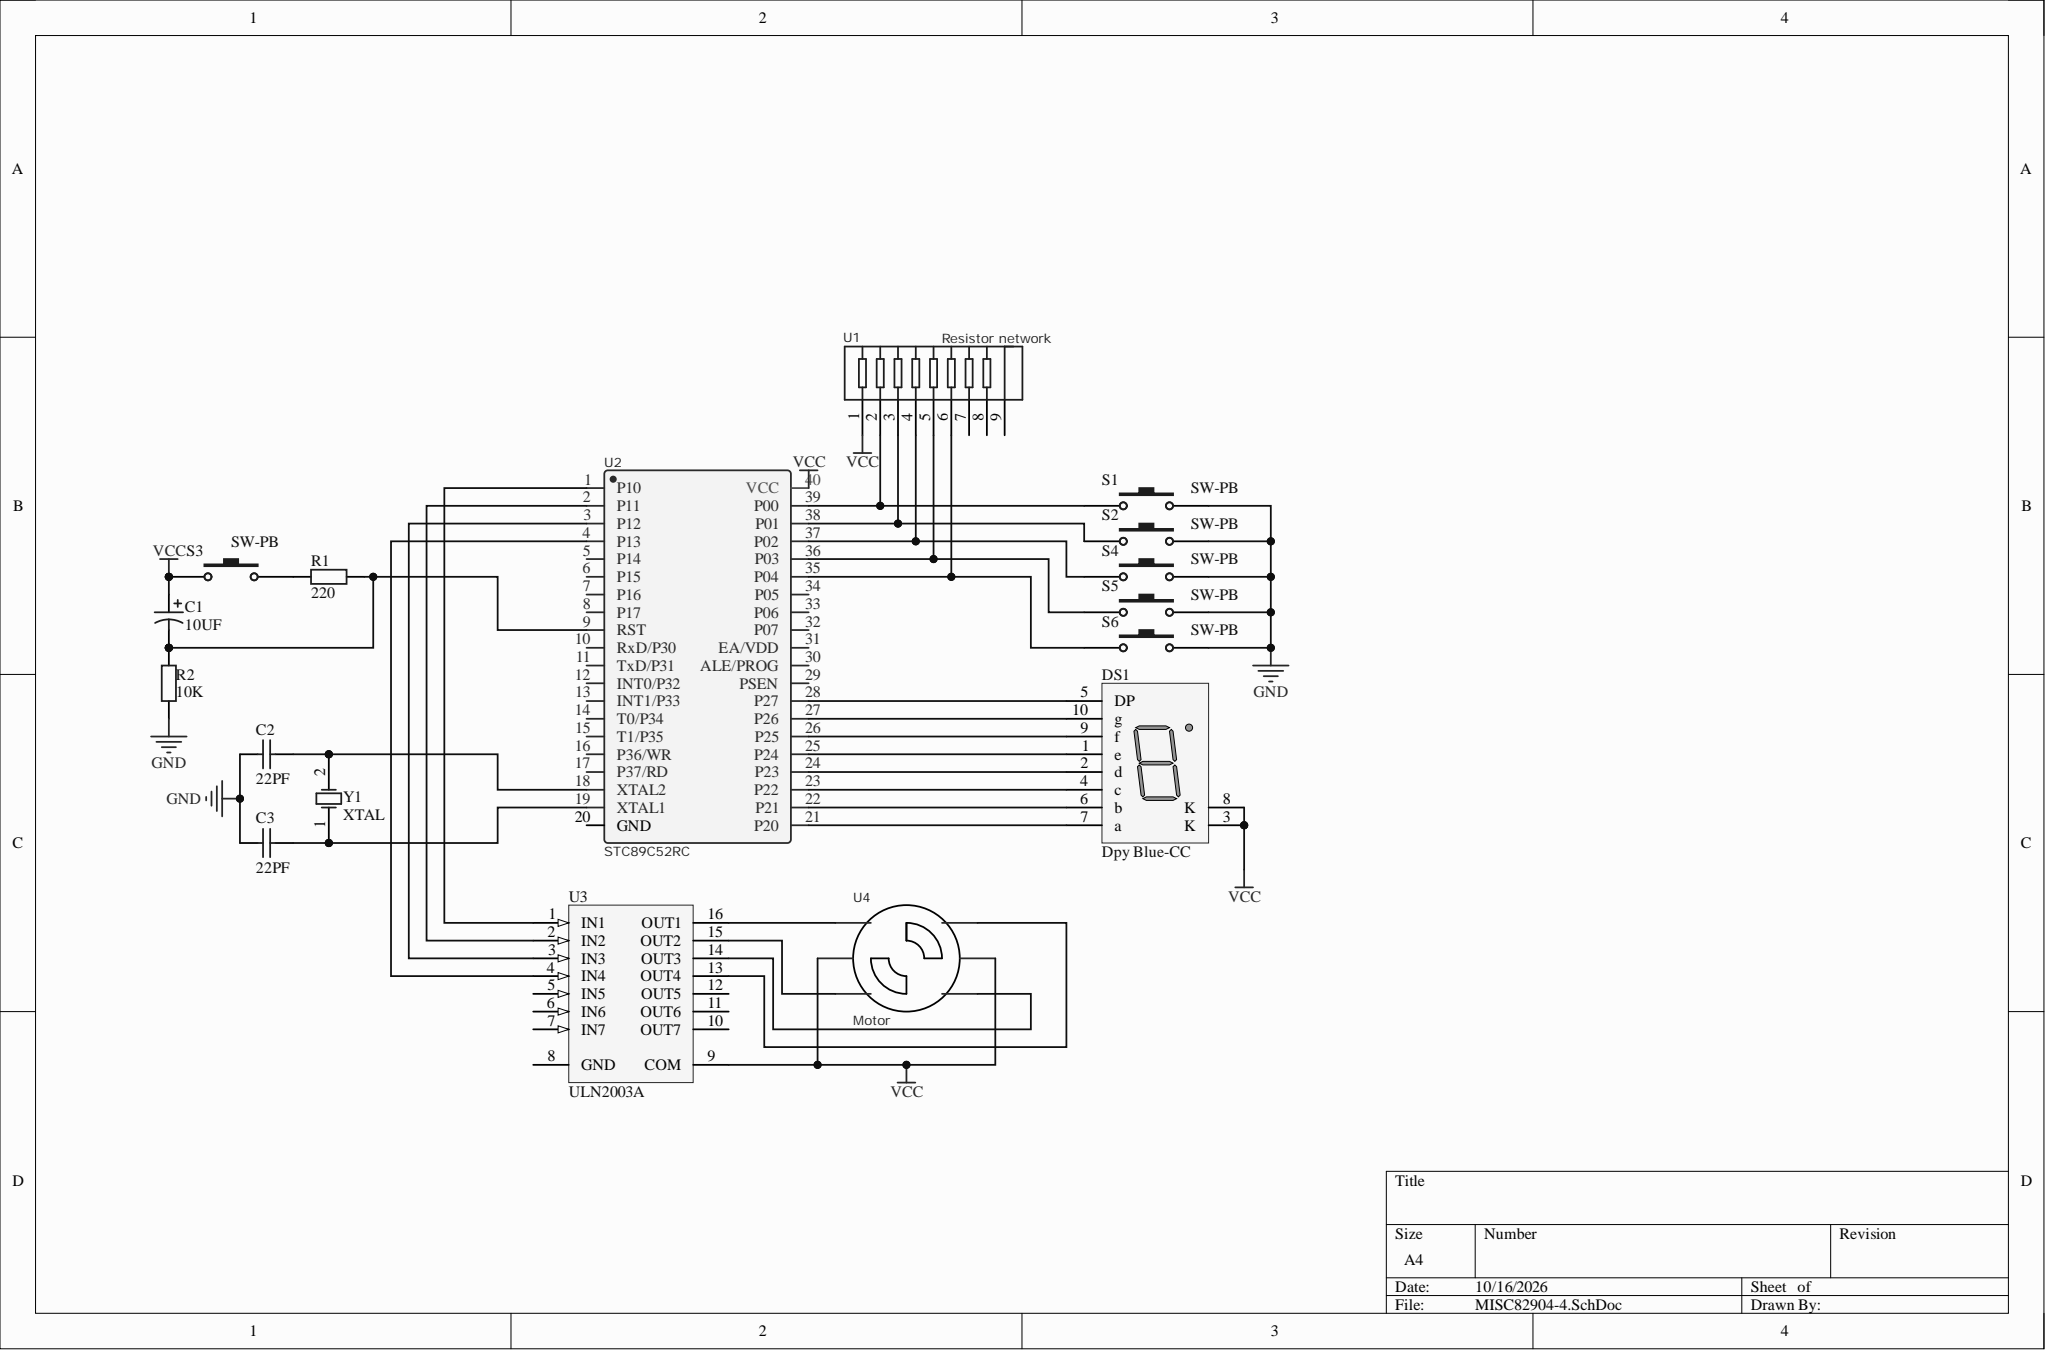Circuit board | Altium Designer | 17 parts | 27 nets
Bill of materials:
Comment,Description,Designator,Footprint,LibRef,Quantity
"10UF","Polarized Capacitor (Radial)","C1","RB7.6-15","Cap Pol1","1"
"22PF","Capacitor","C2, C3","RAD-0.3","Cap","2"
"Dpy Blue-CC","14.2 mm General Purpose Blue 7-Segment Display: CC, RH DP, Gray Surface","DS1","H","Dpy Blue-CC","1"
"220","Resistor","R1","AXIAL-0.4","Res2","1"
"10K","Resistor","R2","AXIAL-0.4","Res2","1"
"SW-PB","Switch","S1, S2, S3, S4, S5, S6","SPST-2","SW-PB","6"
"Resistor network","","U1","paizu","排阻","1"
"STC89C52RC","","U2","STC89C52RC","STC89C52RC","1"
"ULN2003A","High-Voltage, High-Current Darlington Array","U3","A16","ULN2003A","1"
"Motor","","U4","HDR1X6","电机","1"
"XTAL","Crystal Oscillator","Y1","R38","XTAL","1"
Netlist (Protel format):
[
C1
RB7.6-15
10UF



]
[
C2
RAD-0.3
22PF



]
[
C3
RAD-0.3
22PF



]
[
DS1
H
Dpy Blue-CC



]
[
R1
AXIAL-0.4
220



]
[
R2
AXIAL-0.4
10K



]
[
S1
SPST-2
SW-PB



]
[
S2
SPST-2
SW-PB



]
[
S3
SPST-2
SW-PB



]
[
S4
SPST-2
SW-PB



]
[
S5
SPST-2
SW-PB



]
[
S6
SPST-2
SW-PB



]
[
U1
paizu
Resistor network



]
[
U2
STC89C52RC
STC89C52RC



]
[
U3
A16
ULN2003A



]
[
U4
HDR1X6
Motor



]
[
Y1
R38
XTAL



]
(
VCC
C1-1
DS1-3
DS1-8
S3-1
U1-1
U2-40
U3-9
U4-3
U4-5
)
(
NetU3_16
U3-16
U4-1
)
(
NetU3_15
U3-15
U4-2
)
(
NetU3_14
U3-14
U4-6
)
(
NetU3_13
U3-13
U4-4
)
(
NetU2_4
U2-4
U3-4
)
(
NetU2_3
U2-3
U3-3
)
(
NetU2_2
U2-2
U3-2
)
(
NetU2_1
U2-1
U3-1
)
(
NetS6_1
S6-1
U1-6
U2-35
)
(
NetS5_1
S5-1
U1-5
U2-36
)
(
NetS4_1
S4-1
U1-4
U2-37
)
(
NetS2_1
S2-1
U1-3
U2-38
)
(
NetS1_1
S1-1
U1-2
U2-39
)
(
NetR1_2
R1-2
S3-2
)
(
NetDS1_10
DS1-10
U2-27
)
(
NetDS1_9
DS1-9
U2-26
)
(
NetDS1_7
DS1-7
U2-21
)
(
NetDS1_6
DS1-6
U2-22
)
(
NetDS1_5
DS1-5
U2-28
)
(
NetDS1_4
DS1-4
U2-23
)
(
NetDS1_2
DS1-2
U2-24
)
(
NetDS1_1
DS1-1
U2-25
)
(
NetC3_2
C3-2
U2-19
Y1-1
)
(
NetC2_2
C2-2
U2-18
Y1-2
)
(
NetC1_2
C1-2
R1-1
R2-2
U2-9
)
(
GND
C2-1
C3-1
R2-1
S1-2
S2-2
S4-2
S5-2
S6-2
)